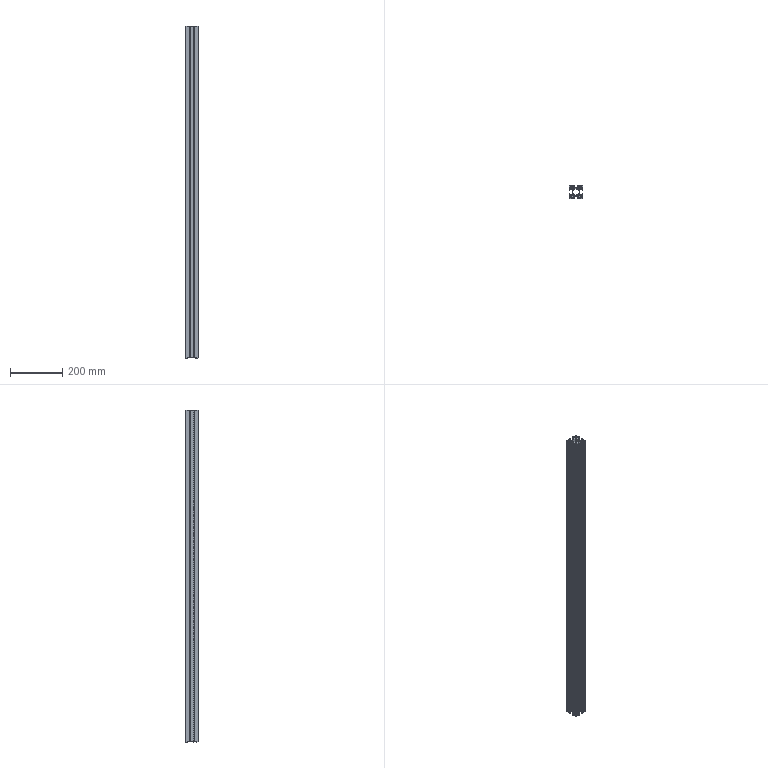Part | STEP file | 46A-00006CC11-1270mm | 1 solid | 142 faces | box 50 x 50 x 1270 mm | volume 746115 mm3 | cylinder 84 | plane 58 | commonest cylinder face diameters 1 x24 4 x24 1.5 x16 3.7 x8 6.7 x8 2 x4